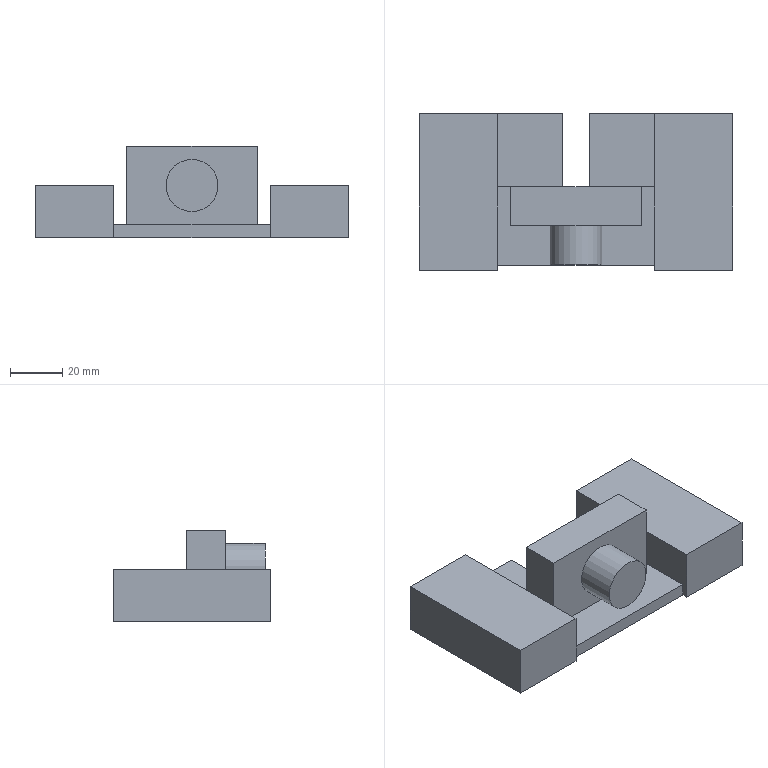Part | STEP file | duishubandingweicao | 3 solids | 32 faces | box 120 x 60 x 35 mm | volume 115212 mm3 | plane 31 | cylinder 1 | commonest cylinder face diameters 20 x1